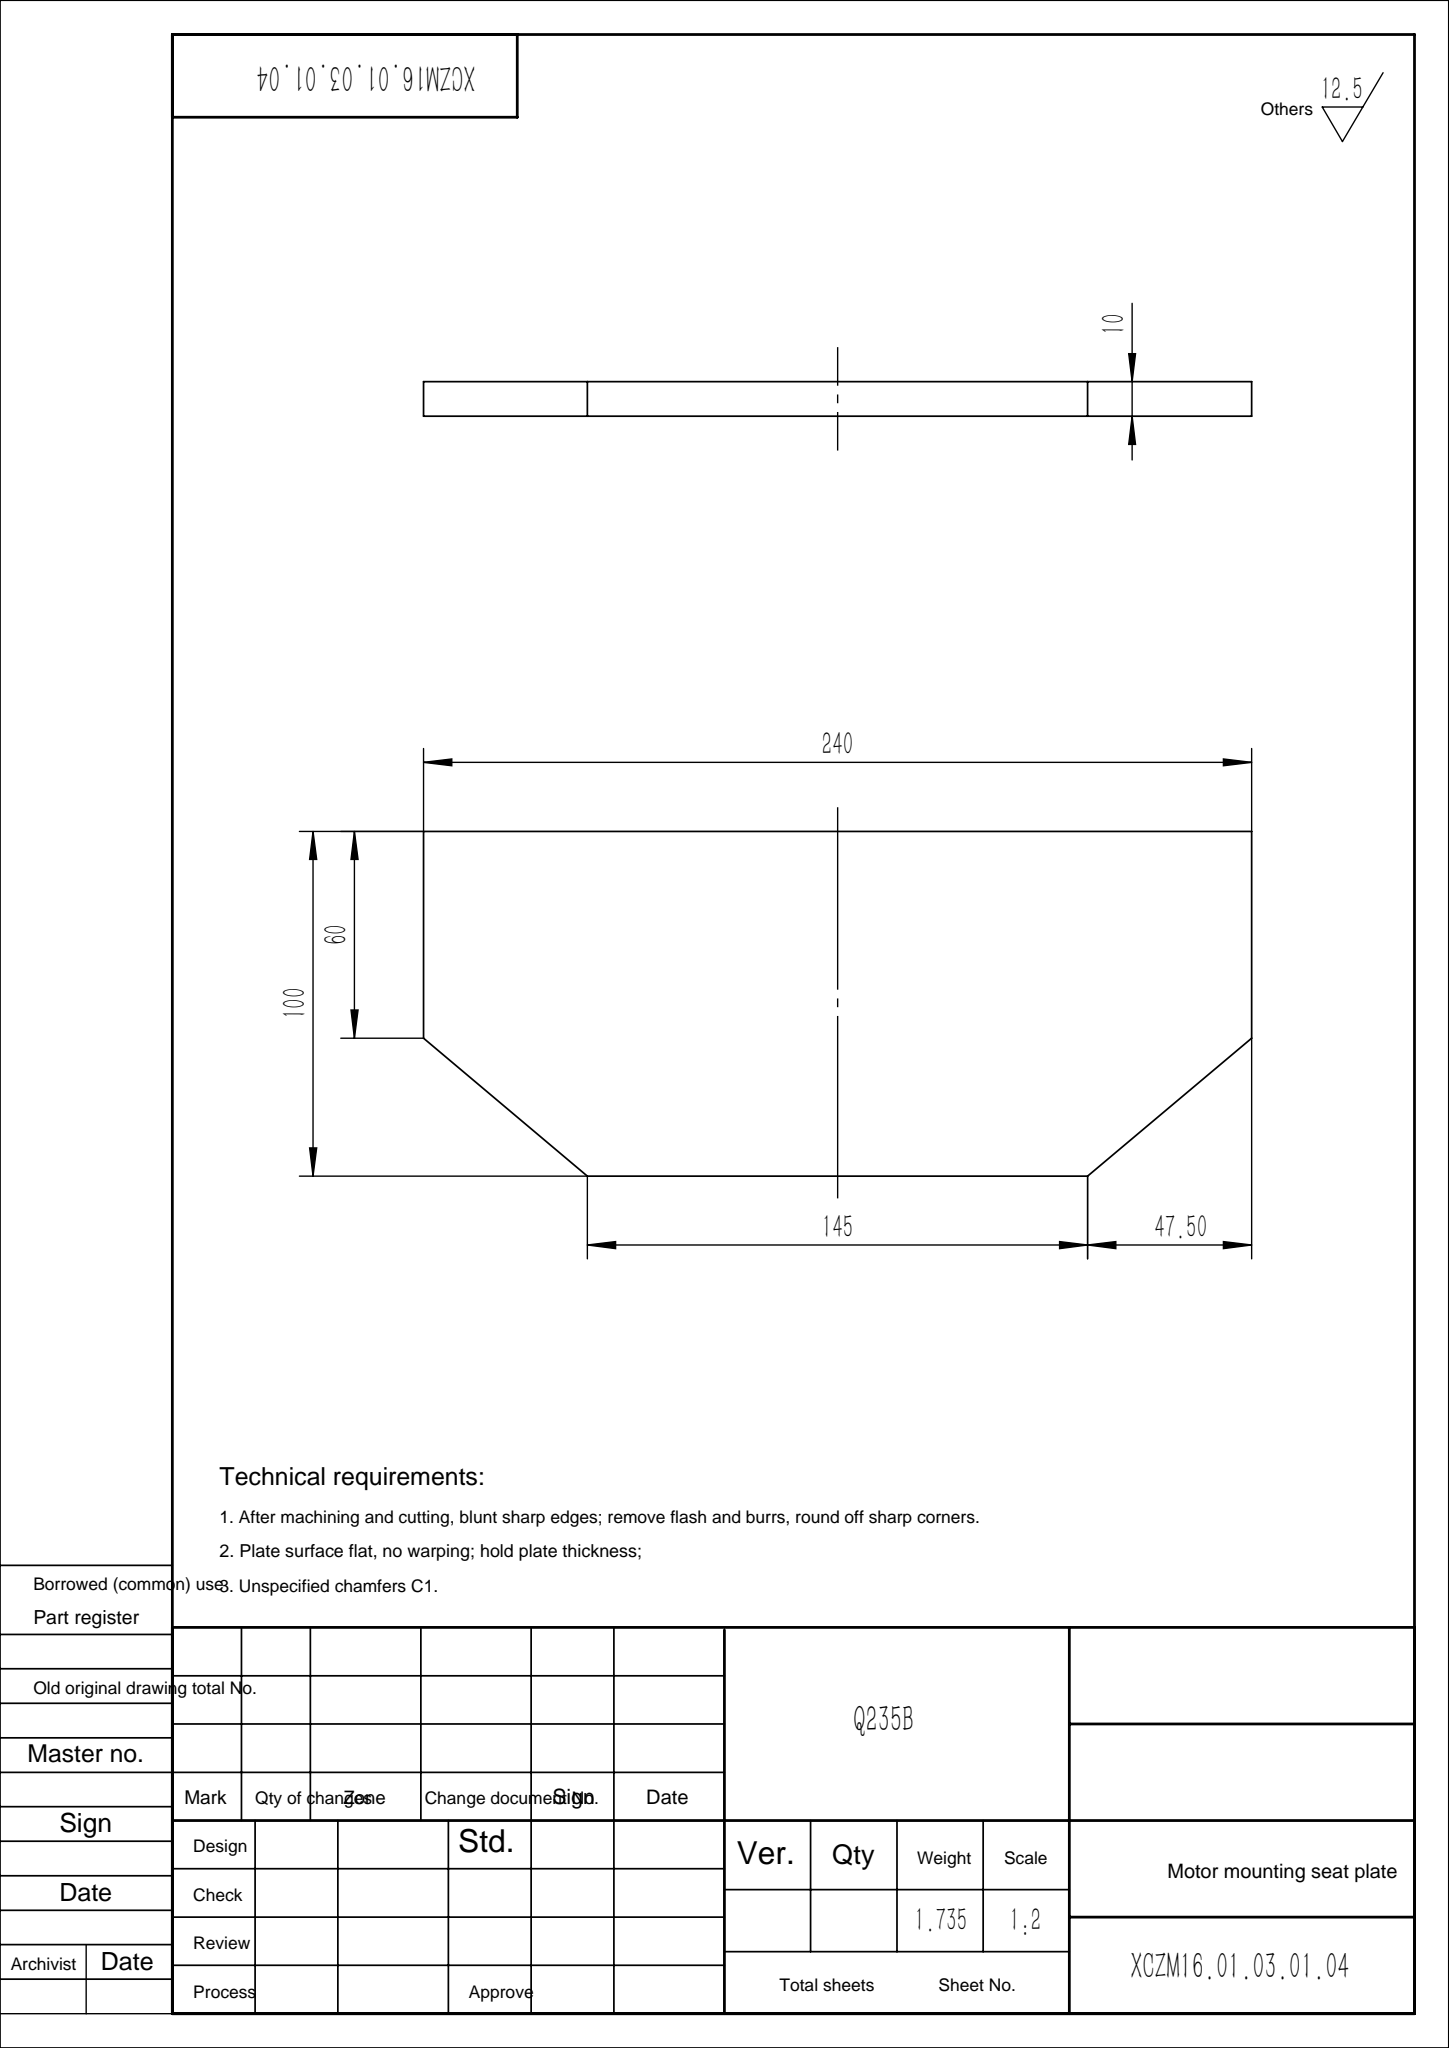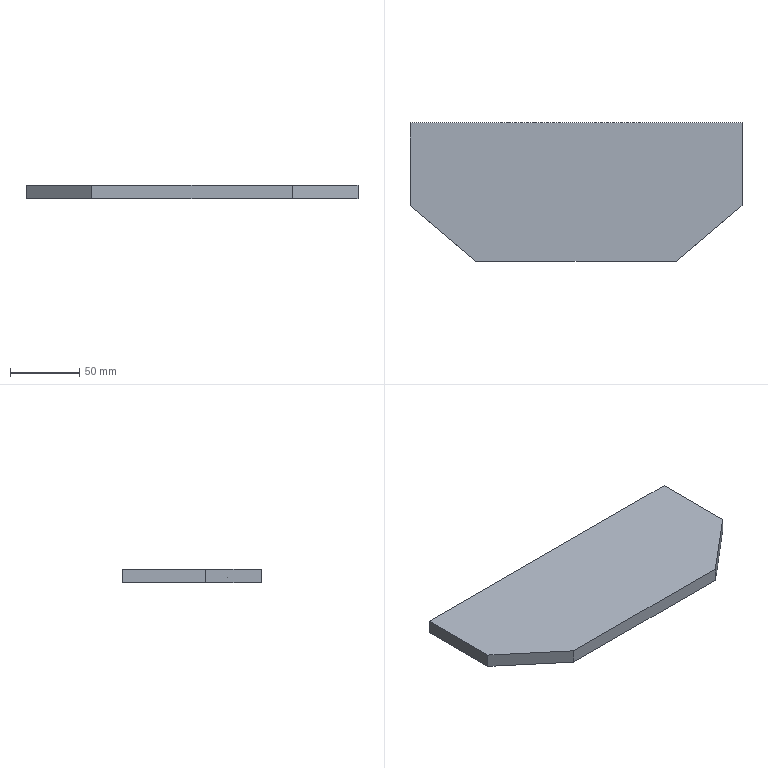Part | SolidWorks | features Extrusion 1 | 1 solid | 8 faces | box 240 x 100 x 10 mm | volume 221000 mm3 | plane 8
STEP:
#1=CARTESIAN_POINT('',(-120.,0.,0.));
#2=VERTEX_POINT('',#1);
#3=CARTESIAN_POINT('',(-120.,-60.,0.));
#4=VERTEX_POINT('',#3);
#5=CARTESIAN_POINT('',(-120.,0.,0.));
#6=DIRECTION('',(0.,-1.,0.));
#7=VECTOR('',#6,1000.);
#8=LINE('',#5,#7);
#9=EDGE_CURVE('',#2,#4,#8,.T.);
#10=ORIENTED_EDGE('',*,*,#9,.T.);
#11=CARTESIAN_POINT('',(-120.,-60.,10.));
#12=VERTEX_POINT('',#11);
#13=CARTESIAN_POINT('',(-120.,-60.,10.));
#14=DIRECTION('',(0.,0.,-1.));
#15=VECTOR('',#14,1000.);
#16=LINE('',#13,#15);
#17=EDGE_CURVE('',#12,#4,#16,.T.);
#18=ORIENTED_EDGE('',*,*,#17,.F.);
#19=CARTESIAN_POINT('',(-120.,0.,10.));
#20=VERTEX_POINT('',#19);
#21=CARTESIAN_POINT('',(-120.,0.,10.));
#22=DIRECTION('',(0.,-1.,0.));
#23=VECTOR('',#22,1000.);
#24=LINE('',#21,#23);
#25=EDGE_CURVE('',#20,#12,#24,.T.);
#26=ORIENTED_EDGE('',*,*,#25,.F.);
#27=CARTESIAN_POINT('',(-120.,0.,10.));
#28=DIRECTION('',(0.,0.,-1.));
#29=VECTOR('',#28,1000.);
#30=LINE('',#27,#29);
#31=EDGE_CURVE('',#20,#2,#30,.T.);
#32=ORIENTED_EDGE('',*,*,#31,.T.);
#33=EDGE_LOOP('',(#10,#18,#26,#32));
#34=FACE_OUTER_BOUND('',#33,.T.);
#35=CARTESIAN_POINT('',(-120.,0.,10.));
#36=DIRECTION('',(1.,0.,0.));
#37=DIRECTION('',(0.,1.,0.));
#38=AXIS2_PLACEMENT_3D('',#35,#36,#37);
#39=PLANE('',#38);
#40=ADVANCED_FACE('',(#34),#39,.F.);
#41=CARTESIAN_POINT('',(-72.5,-100.,0.));
#42=VERTEX_POINT('',#41);
#43=CARTESIAN_POINT('',(-120.,-60.,0.));
#44=DIRECTION('',(0.7649,-0.6441,0.));
#45=VECTOR('',#44,1000.);
#46=LINE('',#43,#45);
#47=EDGE_CURVE('',#4,#42,#46,.T.);
#48=ORIENTED_EDGE('',*,*,#47,.T.);
#49=CARTESIAN_POINT('',(-72.5,-100.,10.));
#50=VERTEX_POINT('',#49);
#51=CARTESIAN_POINT('',(-72.5,-100.,10.));
#52=DIRECTION('',(0.,0.,-1.));
#53=VECTOR('',#52,1000.);
#54=LINE('',#51,#53);
#55=EDGE_CURVE('',#50,#42,#54,.T.);
#56=ORIENTED_EDGE('',*,*,#55,.F.);
#57=CARTESIAN_POINT('',(-120.,-60.,10.));
#58=DIRECTION('',(0.7649,-0.6441,0.));
#59=VECTOR('',#58,1000.);
#60=LINE('',#57,#59);
#61=EDGE_CURVE('',#12,#50,#60,.T.);
#62=ORIENTED_EDGE('',*,*,#61,.F.);
#63=ORIENTED_EDGE('',*,*,#17,.T.);
#64=EDGE_LOOP('',(#48,#56,#62,#63));
#65=FACE_OUTER_BOUND('',#64,.T.);
#66=CARTESIAN_POINT('',(-120.,-60.,10.));
#67=DIRECTION('',(0.6441,0.7649,0.));
#68=DIRECTION('',(-0.7649,0.6441,0.));
#69=AXIS2_PLACEMENT_3D('',#66,#67,#68);
#70=PLANE('',#69);
#71=ADVANCED_FACE('',(#65),#70,.F.);
#72=CARTESIAN_POINT('',(72.5,-100.,0.));
#73=VERTEX_POINT('',#72);
#74=CARTESIAN_POINT('',(-72.5,-100.,0.));
#75=DIRECTION('',(1.,0.,0.));
#76=VECTOR('',#75,1000.);
#77=LINE('',#74,#76);
#78=EDGE_CURVE('',#42,#73,#77,.T.);
#79=ORIENTED_EDGE('',*,*,#78,.T.);
#80=CARTESIAN_POINT('',(72.5,-100.,10.));
#81=VERTEX_POINT('',#80);
#82=CARTESIAN_POINT('',(72.5,-100.,10.));
#83=DIRECTION('',(0.,0.,-1.));
#84=VECTOR('',#83,1000.);
#85=LINE('',#82,#84);
#86=EDGE_CURVE('',#81,#73,#85,.T.);
#87=ORIENTED_EDGE('',*,*,#86,.F.);
#88=CARTESIAN_POINT('',(-72.5,-100.,10.));
#89=DIRECTION('',(1.,0.,0.));
#90=VECTOR('',#89,1000.);
#91=LINE('',#88,#90);
#92=EDGE_CURVE('',#50,#81,#91,.T.);
#93=ORIENTED_EDGE('',*,*,#92,.F.);
#94=ORIENTED_EDGE('',*,*,#55,.T.);
#95=EDGE_LOOP('',(#79,#87,#93,#94));
#96=FACE_OUTER_BOUND('',#95,.T.);
#97=CARTESIAN_POINT('',(-72.5,-100.,10.));
#98=DIRECTION('',(0.,1.,0.));
#99=DIRECTION('',(0.,0.,1.));
#100=AXIS2_PLACEMENT_3D('',#97,#98,#99);
#101=PLANE('',#100);
#102=ADVANCED_FACE('',(#96),#101,.F.);
#103=CARTESIAN_POINT('',(120.,-60.,0.));
#104=VERTEX_POINT('',#103);
#105=CARTESIAN_POINT('',(120.,-60.,0.));
#106=DIRECTION('',(0.7649,0.6441,0.));
#107=VECTOR('',#106,1000.);
#108=LINE('',#105,#107);
#109=EDGE_CURVE('',#73,#104,#108,.T.);
#110=ORIENTED_EDGE('',*,*,#109,.T.);
#111=CARTESIAN_POINT('',(120.,-60.,10.));
#112=VERTEX_POINT('',#111);
#113=CARTESIAN_POINT('',(120.,-60.,10.));
#114=DIRECTION('',(0.,0.,-1.));
#115=VECTOR('',#114,1000.);
#116=LINE('',#113,#115);
#117=EDGE_CURVE('',#112,#104,#116,.T.);
#118=ORIENTED_EDGE('',*,*,#117,.F.);
#119=CARTESIAN_POINT('',(120.,-60.,10.));
#120=DIRECTION('',(0.7649,0.6441,0.));
#121=VECTOR('',#120,1000.);
#122=LINE('',#119,#121);
#123=EDGE_CURVE('',#81,#112,#122,.T.);
#124=ORIENTED_EDGE('',*,*,#123,.F.);
#125=ORIENTED_EDGE('',*,*,#86,.T.);
#126=EDGE_LOOP('',(#110,#118,#124,#125));
#127=FACE_OUTER_BOUND('',#126,.T.);
#128=CARTESIAN_POINT('',(120.,-60.,10.));
#129=DIRECTION('',(-0.6441,0.7649,0.));
#130=DIRECTION('',(-0.7649,-0.6441,0.));
#131=AXIS2_PLACEMENT_3D('',#128,#129,#130);
#132=PLANE('',#131);
#133=ADVANCED_FACE('',(#127),#132,.F.);
#134=CARTESIAN_POINT('',(120.,0.,0.));
#135=VERTEX_POINT('',#134);
#136=CARTESIAN_POINT('',(120.,0.,0.));
#137=DIRECTION('',(0.,1.,0.));
#138=VECTOR('',#137,1000.);
#139=LINE('',#136,#138);
#140=EDGE_CURVE('',#104,#135,#139,.T.);
#141=ORIENTED_EDGE('',*,*,#140,.T.);
#142=CARTESIAN_POINT('',(120.,0.,10.));
#143=VERTEX_POINT('',#142);
#144=CARTESIAN_POINT('',(120.,0.,10.));
#145=DIRECTION('',(0.,0.,-1.));
#146=VECTOR('',#145,1000.);
#147=LINE('',#144,#146);
#148=EDGE_CURVE('',#143,#135,#147,.T.);
#149=ORIENTED_EDGE('',*,*,#148,.F.);
#150=CARTESIAN_POINT('',(120.,0.,10.));
#151=DIRECTION('',(0.,1.,0.));
#152=VECTOR('',#151,1000.);
#153=LINE('',#150,#152);
#154=EDGE_CURVE('',#112,#143,#153,.T.);
#155=ORIENTED_EDGE('',*,*,#154,.F.);
#156=ORIENTED_EDGE('',*,*,#117,.T.);
#157=EDGE_LOOP('',(#141,#149,#155,#156));
#158=FACE_OUTER_BOUND('',#157,.T.);
#159=CARTESIAN_POINT('',(120.,0.,10.));
#160=DIRECTION('',(-1.,0.,0.));
#161=DIRECTION('',(0.,-1.,0.));
#162=AXIS2_PLACEMENT_3D('',#159,#160,#161);
#163=PLANE('',#162);
#164=ADVANCED_FACE('',(#158),#163,.F.);
#165=CARTESIAN_POINT('',(120.,0.,0.));
#166=DIRECTION('',(-1.,0.,0.));
#167=VECTOR('',#166,1000.);
#168=LINE('',#165,#167);
#169=EDGE_CURVE('',#135,#2,#168,.T.);
#170=ORIENTED_EDGE('',*,*,#169,.T.);
#171=ORIENTED_EDGE('',*,*,#31,.F.);
#172=CARTESIAN_POINT('',(120.,0.,10.));
#173=DIRECTION('',(-1.,0.,0.));
#174=VECTOR('',#173,1000.);
#175=LINE('',#172,#174);
#176=EDGE_CURVE('',#143,#20,#175,.T.);
#177=ORIENTED_EDGE('',*,*,#176,.F.);
#178=ORIENTED_EDGE('',*,*,#148,.T.);
#179=EDGE_LOOP('',(#170,#171,#177,#178));
#180=FACE_OUTER_BOUND('',#179,.T.);
#181=CARTESIAN_POINT('',(120.,0.,10.));
#182=DIRECTION('',(0.,-1.,0.));
#183=DIRECTION('',(0.,0.,-1.));
#184=AXIS2_PLACEMENT_3D('',#181,#182,#183);
#185=PLANE('',#184);
#186=ADVANCED_FACE('',(#180),#185,.F.);
#187=ORIENTED_EDGE('',*,*,#25,.T.);
#188=ORIENTED_EDGE('',*,*,#61,.T.);
#189=ORIENTED_EDGE('',*,*,#92,.T.);
#190=ORIENTED_EDGE('',*,*,#123,.T.);
#191=ORIENTED_EDGE('',*,*,#154,.T.);
#192=ORIENTED_EDGE('',*,*,#176,.T.);
#193=EDGE_LOOP('',(#187,#188,#189,#190,#191,#192));
#194=FACE_OUTER_BOUND('',#193,.T.);
#195=CARTESIAN_POINT('',(0.,0.,10.));
#196=DIRECTION('',(0.,0.,1.));
#197=DIRECTION('',(1.,0.,0.));
#198=AXIS2_PLACEMENT_3D('',#195,#196,#197);
#199=PLANE('',#198);
#200=ADVANCED_FACE('',(#194),#199,.T.);
#201=ORIENTED_EDGE('',*,*,#9,.F.);
#202=ORIENTED_EDGE('',*,*,#169,.F.);
#203=ORIENTED_EDGE('',*,*,#140,.F.);
#204=ORIENTED_EDGE('',*,*,#109,.F.);
#205=ORIENTED_EDGE('',*,*,#78,.F.);
#206=ORIENTED_EDGE('',*,*,#47,.F.);
#207=EDGE_LOOP('',(#201,#202,#203,#204,#205,#206));
#208=FACE_OUTER_BOUND('',#207,.T.);
#209=CARTESIAN_POINT('',(0.,0.,0.));
#210=DIRECTION('',(0.,0.,1.));
#211=DIRECTION('',(1.,0.,0.));
#212=AXIS2_PLACEMENT_3D('',#209,#210,#211);
#213=PLANE('',#212);
#214=ADVANCED_FACE('',(#208),#213,.F.);
#215=CLOSED_SHELL('',(#40,#71,#102,#133,#164,#186,#200,#214));
#216=MANIFOLD_SOLID_BREP('',#215);
#217=CARTESIAN_POINT('',(0.,0.,0.));
#218=DIRECTION('',(0.,0.,1.));
#219=DIRECTION('',(1.,0.,0.));
#220=AXIS2_PLACEMENT_3D('',#217,#218,#219);
#221=(LENGTH_UNIT()NAMED_UNIT(*)SI_UNIT(.MILLI.,.METRE.));
#222=UNCERTAINTY_MEASURE_WITH_UNIT(LENGTH_MEASURE(0.00001),#221,'','');
#223=(NAMED_UNIT(*)PLANE_ANGLE_UNIT()SI_UNIT($,.RADIAN.));
#224=(NAMED_UNIT(*)SI_UNIT($,.STERADIAN.)SOLID_ANGLE_UNIT());
#225=(GEOMETRIC_REPRESENTATION_CONTEXT(3)GLOBAL_UNCERTAINTY_ASSIGNED_CONTEXT((#222))GLOBAL_UNIT_ASSIGNED_CONTEXT((#221,#223,#224))REPRESENTATION_CONTEXT('',''));
#226=ADVANCED_BREP_SHAPE_REPRESENTATION('',(#216,#220),#225);